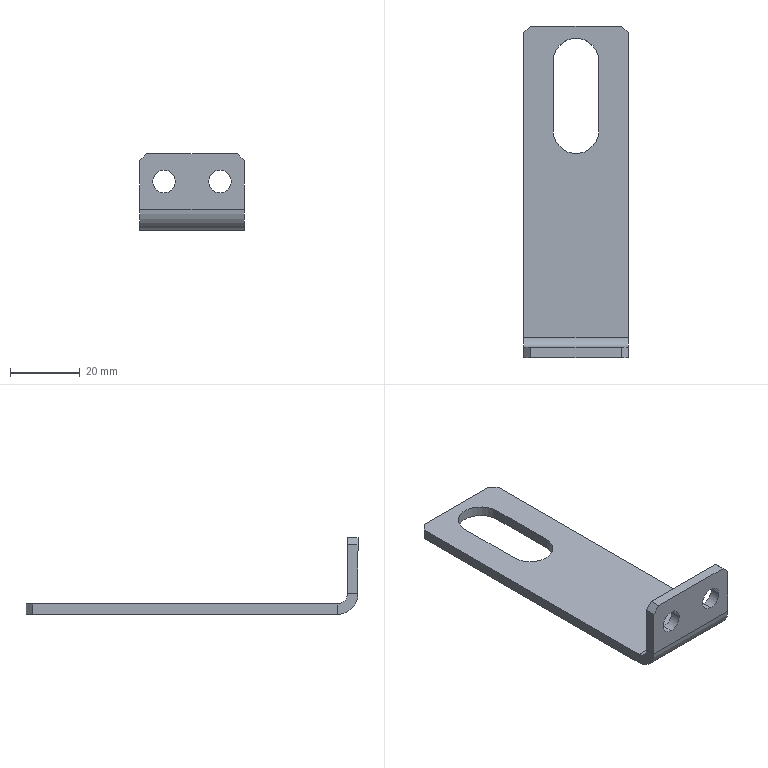Part | SolidWorks | features ICE 2, Chamfer 1, EdgeFlange 1, FlatPattern 1, SMBaseFlange 1, SheetMetal 1 | 1 solid | 26 faces | box 30 x 95 x 22 mm | volume 8685 mm3 | plane 18 | cylinder 8 | commonest cylinder face diameters 6.5 x4 13 x2 6 x1 12 x1
STEP:
#1=CARTESIAN_POINT('',(-8.,-47.5,14.25));
#2=VERTEX_POINT('',#1);
#3=CARTESIAN_POINT('',(-8.,-47.5,7.75));
#4=VERTEX_POINT('',#3);
#5=CARTESIAN_POINT('',(-8.,-47.5,11.));
#6=DIRECTION('',(0.,-1.,0.));
#7=DIRECTION('',(0.,0.,-1.));
#8=AXIS2_PLACEMENT_3D('',#5,#6,#7);
#9=CIRCLE('',#8,3.25);
#10=EDGE_CURVE('',#2,#4,#9,.T.);
#11=ORIENTED_EDGE('',*,*,#10,.T.);
#12=CARTESIAN_POINT('',(-8.,-44.5,7.75));
#13=VERTEX_POINT('',#12);
#14=CARTESIAN_POINT('',(-8.,-54.5,7.75));
#15=DIRECTION('',(0.,1.,0.));
#16=VECTOR('',#15,1000.);
#17=LINE('',#14,#16);
#18=EDGE_CURVE('',#4,#13,#17,.T.);
#19=ORIENTED_EDGE('',*,*,#18,.T.);
#20=CARTESIAN_POINT('',(-8.,-44.5,14.25));
#21=VERTEX_POINT('',#20);
#22=CARTESIAN_POINT('',(-8.,-44.5,11.));
#23=DIRECTION('',(0.,1.,0.));
#24=DIRECTION('',(0.,0.,1.));
#25=AXIS2_PLACEMENT_3D('',#22,#23,#24);
#26=CIRCLE('',#25,3.25);
#27=EDGE_CURVE('',#13,#21,#26,.T.);
#28=ORIENTED_EDGE('',*,*,#27,.T.);
#29=CARTESIAN_POINT('',(-8.,-54.5,14.25));
#30=DIRECTION('',(0.,1.,0.));
#31=VECTOR('',#30,1000.);
#32=LINE('',#29,#31);
#33=EDGE_CURVE('',#2,#21,#32,.T.);
#34=ORIENTED_EDGE('',*,*,#33,.F.);
#35=EDGE_LOOP('',(#11,#19,#28,#34));
#36=FACE_OUTER_BOUND('',#35,.T.);
#37=CARTESIAN_POINT('',(-8.,-54.5,11.));
#38=DIRECTION('',(0.,1.,0.));
#39=DIRECTION('',(0.,0.,1.));
#40=AXIS2_PLACEMENT_3D('',#37,#38,#39);
#41=CYLINDRICAL_SURFACE('',#40,3.25);
#42=ADVANCED_FACE('',(#36),#41,.F.);
#43=CARTESIAN_POINT('',(8.,-47.5,14.25));
#44=VERTEX_POINT('',#43);
#45=CARTESIAN_POINT('',(8.,-47.5,7.75));
#46=VERTEX_POINT('',#45);
#47=CARTESIAN_POINT('',(8.,-47.5,11.));
#48=DIRECTION('',(0.,-1.,0.));
#49=DIRECTION('',(0.,0.,-1.));
#50=AXIS2_PLACEMENT_3D('',#47,#48,#49);
#51=CIRCLE('',#50,3.25);
#52=EDGE_CURVE('',#44,#46,#51,.T.);
#53=ORIENTED_EDGE('',*,*,#52,.T.);
#54=CARTESIAN_POINT('',(8.,-44.5,7.75));
#55=VERTEX_POINT('',#54);
#56=CARTESIAN_POINT('',(8.,-54.5,7.75));
#57=DIRECTION('',(0.,1.,0.));
#58=VECTOR('',#57,1000.);
#59=LINE('',#56,#58);
#60=EDGE_CURVE('',#46,#55,#59,.T.);
#61=ORIENTED_EDGE('',*,*,#60,.T.);
#62=CARTESIAN_POINT('',(8.,-44.5,14.25));
#63=VERTEX_POINT('',#62);
#64=CARTESIAN_POINT('',(8.,-44.5,11.));
#65=DIRECTION('',(0.,1.,0.));
#66=DIRECTION('',(0.,0.,1.));
#67=AXIS2_PLACEMENT_3D('',#64,#65,#66);
#68=CIRCLE('',#67,3.25);
#69=EDGE_CURVE('',#55,#63,#68,.T.);
#70=ORIENTED_EDGE('',*,*,#69,.T.);
#71=CARTESIAN_POINT('',(8.,-54.5,14.25));
#72=DIRECTION('',(0.,1.,0.));
#73=VECTOR('',#72,1000.);
#74=LINE('',#71,#73);
#75=EDGE_CURVE('',#44,#63,#74,.T.);
#76=ORIENTED_EDGE('',*,*,#75,.F.);
#77=EDGE_LOOP('',(#53,#61,#70,#76));
#78=FACE_OUTER_BOUND('',#77,.T.);
#79=CARTESIAN_POINT('',(8.,-54.5,11.));
#80=DIRECTION('',(0.,1.,0.));
#81=DIRECTION('',(0.,0.,1.));
#82=AXIS2_PLACEMENT_3D('',#79,#80,#81);
#83=CYLINDRICAL_SURFACE('',#82,3.25);
#84=ADVANCED_FACE('',(#78),#83,.F.);
#85=CARTESIAN_POINT('',(15.,-41.5,-3.));
#86=VERTEX_POINT('',#85);
#87=CARTESIAN_POINT('',(15.,45.5,-3.));
#88=VERTEX_POINT('',#87);
#89=CARTESIAN_POINT('',(15.,-47.5,-3.));
#90=DIRECTION('',(0.,1.,0.));
#91=VECTOR('',#90,1000.);
#92=LINE('',#89,#91);
#93=EDGE_CURVE('',#86,#88,#92,.T.);
#94=ORIENTED_EDGE('',*,*,#93,.T.);
#95=CARTESIAN_POINT('',(15.,45.5,0.));
#96=VERTEX_POINT('',#95);
#97=CARTESIAN_POINT('',(15.,45.5,-3.));
#98=DIRECTION('',(0.,0.,1.));
#99=VECTOR('',#98,1000.);
#100=LINE('',#97,#99);
#101=EDGE_CURVE('',#88,#96,#100,.T.);
#102=ORIENTED_EDGE('',*,*,#101,.T.);
#103=CARTESIAN_POINT('',(15.,-41.5,0.));
#104=VERTEX_POINT('',#103);
#105=CARTESIAN_POINT('',(15.,-47.5,0.));
#106=DIRECTION('',(0.,1.,0.));
#107=VECTOR('',#106,1000.);
#108=LINE('',#105,#107);
#109=EDGE_CURVE('',#104,#96,#108,.T.);
#110=ORIENTED_EDGE('',*,*,#109,.F.);
#111=CARTESIAN_POINT('',(15.,-41.5,0.));
#112=DIRECTION('',(0.,0.,-1.));
#113=VECTOR('',#112,1000.);
#114=LINE('',#111,#113);
#115=EDGE_CURVE('',#104,#86,#114,.T.);
#116=ORIENTED_EDGE('',*,*,#115,.T.);
#117=EDGE_LOOP('',(#94,#102,#110,#116));
#118=FACE_OUTER_BOUND('',#117,.T.);
#119=CARTESIAN_POINT('',(15.,-47.5,-3.));
#120=DIRECTION('',(1.,0.,0.));
#121=DIRECTION('',(0.,0.,-1.));
#122=AXIS2_PLACEMENT_3D('',#119,#120,#121);
#123=PLANE('',#122);
#124=ADVANCED_FACE('',(#118),#123,.T.);
#125=CARTESIAN_POINT('',(6.5,37.5,-3.));
#126=VERTEX_POINT('',#125);
#127=CARTESIAN_POINT('',(-6.5,37.5,-3.));
#128=VERTEX_POINT('',#127);
#129=CARTESIAN_POINT('',(0.,37.5,-3.));
#130=DIRECTION('',(0.,0.,1.));
#131=DIRECTION('',(1.,0.,0.));
#132=AXIS2_PLACEMENT_3D('',#129,#130,#131);
#133=CIRCLE('',#132,6.5);
#134=EDGE_CURVE('',#126,#128,#133,.T.);
#135=ORIENTED_EDGE('',*,*,#134,.T.);
#136=CARTESIAN_POINT('',(-6.5,17.5,-3.));
#137=VERTEX_POINT('',#136);
#138=CARTESIAN_POINT('',(-6.5,37.5,-3.));
#139=DIRECTION('',(0.,-1.,0.));
#140=VECTOR('',#139,1000.);
#141=LINE('',#138,#140);
#142=EDGE_CURVE('',#128,#137,#141,.T.);
#143=ORIENTED_EDGE('',*,*,#142,.T.);
#144=CARTESIAN_POINT('',(6.5,17.5,-3.));
#145=VERTEX_POINT('',#144);
#146=CARTESIAN_POINT('',(0.,17.5,-3.));
#147=DIRECTION('',(0.,0.,1.));
#148=DIRECTION('',(1.,0.,0.));
#149=AXIS2_PLACEMENT_3D('',#146,#147,#148);
#150=CIRCLE('',#149,6.5);
#151=EDGE_CURVE('',#137,#145,#150,.T.);
#152=ORIENTED_EDGE('',*,*,#151,.T.);
#153=CARTESIAN_POINT('',(6.5,37.5,-3.));
#154=DIRECTION('',(0.,1.,0.));
#155=VECTOR('',#154,1000.);
#156=LINE('',#153,#155);
#157=EDGE_CURVE('',#145,#126,#156,.T.);
#158=ORIENTED_EDGE('',*,*,#157,.T.);
#159=EDGE_LOOP('',(#135,#143,#152,#158));
#160=FACE_BOUND('',#159,.T.);
#161=CARTESIAN_POINT('',(13.,47.5,-3.));
#162=VERTEX_POINT('',#161);
#163=CARTESIAN_POINT('',(-13.,47.5,-3.));
#164=VERTEX_POINT('',#163);
#165=CARTESIAN_POINT('',(-15.,47.5,-3.));
#166=DIRECTION('',(-1.,0.,0.));
#167=VECTOR('',#166,1000.);
#168=LINE('',#165,#167);
#169=EDGE_CURVE('',#162,#164,#168,.T.);
#170=ORIENTED_EDGE('',*,*,#169,.F.);
#171=CARTESIAN_POINT('',(30.25,30.25,-3.));
#172=DIRECTION('',(0.7071,-0.7071,0.));
#173=VECTOR('',#172,1000.);
#174=LINE('',#171,#173);
#175=EDGE_CURVE('',#162,#88,#174,.T.);
#176=ORIENTED_EDGE('',*,*,#175,.T.);
#177=ORIENTED_EDGE('',*,*,#93,.F.);
#178=CARTESIAN_POINT('',(-15.,-41.5,-3.));
#179=VERTEX_POINT('',#178);
#180=CARTESIAN_POINT('',(15.,-41.5,-3.));
#181=DIRECTION('',(-1.,0.,0.));
#182=VECTOR('',#181,1000.);
#183=LINE('',#180,#182);
#184=EDGE_CURVE('',#86,#179,#183,.T.);
#185=ORIENTED_EDGE('',*,*,#184,.T.);
#186=CARTESIAN_POINT('',(-15.,45.5,-3.));
#187=VERTEX_POINT('',#186);
#188=CARTESIAN_POINT('',(-15.,-47.5,-3.));
#189=DIRECTION('',(0.,-1.,0.));
#190=VECTOR('',#189,1000.);
#191=LINE('',#188,#190);
#192=EDGE_CURVE('',#187,#179,#191,.T.);
#193=ORIENTED_EDGE('',*,*,#192,.F.);
#194=CARTESIAN_POINT('',(-30.25,30.25,-3.));
#195=DIRECTION('',(0.7071,0.7071,0.));
#196=VECTOR('',#195,1000.);
#197=LINE('',#194,#196);
#198=EDGE_CURVE('',#187,#164,#197,.T.);
#199=ORIENTED_EDGE('',*,*,#198,.T.);
#200=EDGE_LOOP('',(#170,#176,#177,#185,#193,#199));
#201=FACE_OUTER_BOUND('',#200,.T.);
#202=CARTESIAN_POINT('',(0.,0.,-3.));
#203=DIRECTION('',(0.,0.,-1.));
#204=DIRECTION('',(-1.,0.,0.));
#205=AXIS2_PLACEMENT_3D('',#202,#203,#204);
#206=PLANE('',#205);
#207=ADVANCED_FACE('',(#160,#201),#206,.T.);
#208=CARTESIAN_POINT('',(-6.5,37.5,0.));
#209=VERTEX_POINT('',#208);
#210=CARTESIAN_POINT('',(-6.5,17.5,0.));
#211=VERTEX_POINT('',#210);
#212=CARTESIAN_POINT('',(-6.5,37.5,0.));
#213=DIRECTION('',(0.,-1.,0.));
#214=VECTOR('',#213,1000.);
#215=LINE('',#212,#214);
#216=EDGE_CURVE('',#209,#211,#215,.T.);
#217=ORIENTED_EDGE('',*,*,#216,.F.);
#218=CARTESIAN_POINT('',(6.5,37.5,0.));
#219=VERTEX_POINT('',#218);
#220=CARTESIAN_POINT('',(0.,37.5,0.));
#221=DIRECTION('',(0.,0.,1.));
#222=DIRECTION('',(1.,0.,0.));
#223=AXIS2_PLACEMENT_3D('',#220,#221,#222);
#224=CIRCLE('',#223,6.5);
#225=EDGE_CURVE('',#219,#209,#224,.T.);
#226=ORIENTED_EDGE('',*,*,#225,.F.);
#227=CARTESIAN_POINT('',(6.5,17.5,0.));
#228=VERTEX_POINT('',#227);
#229=CARTESIAN_POINT('',(6.5,37.5,0.));
#230=DIRECTION('',(0.,1.,0.));
#231=VECTOR('',#230,1000.);
#232=LINE('',#229,#231);
#233=EDGE_CURVE('',#228,#219,#232,.T.);
#234=ORIENTED_EDGE('',*,*,#233,.F.);
#235=CARTESIAN_POINT('',(0.,17.5,0.));
#236=DIRECTION('',(0.,0.,1.));
#237=DIRECTION('',(1.,0.,0.));
#238=AXIS2_PLACEMENT_3D('',#235,#236,#237);
#239=CIRCLE('',#238,6.5);
#240=EDGE_CURVE('',#211,#228,#239,.T.);
#241=ORIENTED_EDGE('',*,*,#240,.F.);
#242=EDGE_LOOP('',(#217,#226,#234,#241));
#243=FACE_BOUND('',#242,.T.);
#244=ORIENTED_EDGE('',*,*,#109,.T.);
#245=CARTESIAN_POINT('',(13.,47.5,0.));
#246=VERTEX_POINT('',#245);
#247=CARTESIAN_POINT('',(15.,45.5,0.));
#248=DIRECTION('',(-0.7071,0.7071,0.));
#249=VECTOR('',#248,1000.);
#250=LINE('',#247,#249);
#251=EDGE_CURVE('',#96,#246,#250,.T.);
#252=ORIENTED_EDGE('',*,*,#251,.T.);
#253=CARTESIAN_POINT('',(-13.,47.5,0.));
#254=VERTEX_POINT('',#253);
#255=CARTESIAN_POINT('',(-15.,47.5,0.));
#256=DIRECTION('',(-1.,0.,0.));
#257=VECTOR('',#256,1000.);
#258=LINE('',#255,#257);
#259=EDGE_CURVE('',#246,#254,#258,.T.);
#260=ORIENTED_EDGE('',*,*,#259,.T.);
#261=CARTESIAN_POINT('',(-15.,45.5,0.));
#262=VERTEX_POINT('',#261);
#263=CARTESIAN_POINT('',(-13.,47.5,0.));
#264=DIRECTION('',(-0.7071,-0.7071,0.));
#265=VECTOR('',#264,1000.);
#266=LINE('',#263,#265);
#267=EDGE_CURVE('',#254,#262,#266,.T.);
#268=ORIENTED_EDGE('',*,*,#267,.T.);
#269=CARTESIAN_POINT('',(-15.,-41.5,0.));
#270=VERTEX_POINT('',#269);
#271=CARTESIAN_POINT('',(-15.,-47.5,0.));
#272=DIRECTION('',(0.,-1.,0.));
#273=VECTOR('',#272,1000.);
#274=LINE('',#271,#273);
#275=EDGE_CURVE('',#262,#270,#274,.T.);
#276=ORIENTED_EDGE('',*,*,#275,.T.);
#277=CARTESIAN_POINT('',(15.,-41.5,0.));
#278=DIRECTION('',(-1.,0.,0.));
#279=VECTOR('',#278,1000.);
#280=LINE('',#277,#279);
#281=EDGE_CURVE('',#104,#270,#280,.T.);
#282=ORIENTED_EDGE('',*,*,#281,.F.);
#283=EDGE_LOOP('',(#244,#252,#260,#268,#276,#282));
#284=FACE_OUTER_BOUND('',#283,.T.);
#285=CARTESIAN_POINT('',(0.,0.,0.));
#286=DIRECTION('',(0.,0.,-1.));
#287=DIRECTION('',(-1.,0.,0.));
#288=AXIS2_PLACEMENT_3D('',#285,#286,#287);
#289=PLANE('',#288);
#290=ADVANCED_FACE('',(#243,#284),#289,.F.);
#291=ORIENTED_EDGE('',*,*,#275,.F.);
#292=CARTESIAN_POINT('',(-15.,45.5,-3.));
#293=DIRECTION('',(0.,0.,-1.));
#294=VECTOR('',#293,1000.);
#295=LINE('',#292,#294);
#296=EDGE_CURVE('',#262,#187,#295,.T.);
#297=ORIENTED_EDGE('',*,*,#296,.T.);
#298=ORIENTED_EDGE('',*,*,#192,.T.);
#299=CARTESIAN_POINT('',(-15.,-41.5,0.));
#300=DIRECTION('',(0.,0.,-1.));
#301=VECTOR('',#300,1000.);
#302=LINE('',#299,#301);
#303=EDGE_CURVE('',#270,#179,#302,.T.);
#304=ORIENTED_EDGE('',*,*,#303,.F.);
#305=EDGE_LOOP('',(#291,#297,#298,#304));
#306=FACE_OUTER_BOUND('',#305,.T.);
#307=CARTESIAN_POINT('',(-15.,-47.5,-3.));
#308=DIRECTION('',(-1.,0.,0.));
#309=DIRECTION('',(0.,0.,1.));
#310=AXIS2_PLACEMENT_3D('',#307,#308,#309);
#311=PLANE('',#310);
#312=ADVANCED_FACE('',(#306),#311,.T.);
#313=ORIENTED_EDGE('',*,*,#259,.F.);
#314=CARTESIAN_POINT('',(13.,47.5,-3.));
#315=DIRECTION('',(0.,0.,-1.));
#316=VECTOR('',#315,1000.);
#317=LINE('',#314,#316);
#318=EDGE_CURVE('',#246,#162,#317,.T.);
#319=ORIENTED_EDGE('',*,*,#318,.T.);
#320=ORIENTED_EDGE('',*,*,#169,.T.);
#321=CARTESIAN_POINT('',(-13.,47.5,-3.));
#322=DIRECTION('',(0.,0.,1.));
#323=VECTOR('',#322,1000.);
#324=LINE('',#321,#323);
#325=EDGE_CURVE('',#164,#254,#324,.T.);
#326=ORIENTED_EDGE('',*,*,#325,.T.);
#327=EDGE_LOOP('',(#313,#319,#320,#326));
#328=FACE_OUTER_BOUND('',#327,.T.);
#329=CARTESIAN_POINT('',(-15.,47.5,-3.));
#330=DIRECTION('',(0.,1.,0.));
#331=DIRECTION('',(0.,0.,1.));
#332=AXIS2_PLACEMENT_3D('',#329,#330,#331);
#333=PLANE('',#332);
#334=ADVANCED_FACE('',(#328),#333,.T.);
#335=CARTESIAN_POINT('',(-15.,-44.5,3.));
#336=VERTEX_POINT('',#335);
#337=CARTESIAN_POINT('',(-15.,-47.5,3.));
#338=VERTEX_POINT('',#337);
#339=CARTESIAN_POINT('',(-15.,-47.5,3.));
#340=DIRECTION('',(0.,-1.,0.));
#341=VECTOR('',#340,1000.);
#342=LINE('',#339,#341);
#343=EDGE_CURVE('',#336,#338,#342,.T.);
#344=ORIENTED_EDGE('',*,*,#343,.F.);
#345=CARTESIAN_POINT('',(-15.,-41.5,3.));
#346=DIRECTION('',(-1.,0.,0.));
#347=DIRECTION('',(0.,0.,-1.));
#348=AXIS2_PLACEMENT_3D('',#345,#346,#347);
#349=CIRCLE('',#348,3.);
#350=EDGE_CURVE('',#270,#336,#349,.T.);
#351=ORIENTED_EDGE('',*,*,#350,.F.);
#352=ORIENTED_EDGE('',*,*,#303,.T.);
#353=CARTESIAN_POINT('',(-15.,-41.5,3.));
#354=DIRECTION('',(-1.,0.,0.));
#355=DIRECTION('',(0.,0.,-1.));
#356=AXIS2_PLACEMENT_3D('',#353,#354,#355);
#357=CIRCLE('',#356,6.);
#358=EDGE_CURVE('',#179,#338,#357,.T.);
#359=ORIENTED_EDGE('',*,*,#358,.T.);
#360=EDGE_LOOP('',(#344,#351,#352,#359));
#361=FACE_OUTER_BOUND('',#360,.T.);
#362=CARTESIAN_POINT('',(-15.,-41.5,3.));
#363=DIRECTION('',(-1.,0.,0.));
#364=DIRECTION('',(0.,0.,1.));
#365=AXIS2_PLACEMENT_3D('',#362,#363,#364);
#366=PLANE('',#365);
#367=ADVANCED_FACE('',(#361),#366,.T.);
#368=CARTESIAN_POINT('',(15.,-44.5,3.));
#369=VERTEX_POINT('',#368);
#370=CARTESIAN_POINT('',(15.,-41.5,3.));
#371=DIRECTION('',(1.,0.,0.));
#372=DIRECTION('',(0.,0.,-1.));
#373=AXIS2_PLACEMENT_3D('',#370,#371,#372);
#374=CIRCLE('',#373,3.);
#375=EDGE_CURVE('',#369,#104,#374,.T.);
#376=ORIENTED_EDGE('',*,*,#375,.F.);
#377=CARTESIAN_POINT('',(15.,-47.5,3.));
#378=VERTEX_POINT('',#377);
#379=CARTESIAN_POINT('',(15.,-44.5,3.));
#380=DIRECTION('',(0.,-1.,0.));
#381=VECTOR('',#380,1000.);
#382=LINE('',#379,#381);
#383=EDGE_CURVE('',#369,#378,#382,.T.);
#384=ORIENTED_EDGE('',*,*,#383,.T.);
#385=CARTESIAN_POINT('',(15.,-41.5,3.));
#386=DIRECTION('',(1.,0.,0.));
#387=DIRECTION('',(0.,0.,-1.));
#388=AXIS2_PLACEMENT_3D('',#385,#386,#387);
#389=CIRCLE('',#388,6.);
#390=EDGE_CURVE('',#378,#86,#389,.T.);
#391=ORIENTED_EDGE('',*,*,#390,.T.);
#392=ORIENTED_EDGE('',*,*,#115,.F.);
#393=EDGE_LOOP('',(#376,#384,#391,#392));
#394=FACE_OUTER_BOUND('',#393,.T.);
#395=CARTESIAN_POINT('',(15.,-41.5,3.));
#396=DIRECTION('',(-1.,0.,0.));
#397=DIRECTION('',(0.,0.,1.));
#398=AXIS2_PLACEMENT_3D('',#395,#396,#397);
#399=PLANE('',#398);
#400=ADVANCED_FACE('',(#394),#399,.F.);
#401=ORIENTED_EDGE('',*,*,#184,.F.);
#402=ORIENTED_EDGE('',*,*,#390,.F.);
#403=CARTESIAN_POINT('',(0.,-47.5,3.));
#404=DIRECTION('',(1.,0.,0.));
#405=VECTOR('',#404,1000.);
#406=LINE('',#403,#405);
#407=EDGE_CURVE('',#338,#378,#406,.T.);
#408=ORIENTED_EDGE('',*,*,#407,.F.);
#409=ORIENTED_EDGE('',*,*,#358,.F.);
#410=EDGE_LOOP('',(#401,#402,#408,#409));
#411=FACE_OUTER_BOUND('',#410,.T.);
#412=CARTESIAN_POINT('',(15.,-41.5,3.));
#413=DIRECTION('',(1.,0.,0.));
#414=DIRECTION('',(0.,-1.,0.));
#415=AXIS2_PLACEMENT_3D('',#412,#413,#414);
#416=CYLINDRICAL_SURFACE('',#415,6.);
#417=ADVANCED_FACE('',(#411),#416,.T.);
#418=ORIENTED_EDGE('',*,*,#281,.T.);
#419=ORIENTED_EDGE('',*,*,#350,.T.);
#420=CARTESIAN_POINT('',(-15.,-44.5,3.));
#421=DIRECTION('',(1.,0.,0.));
#422=VECTOR('',#421,1000.);
#423=LINE('',#420,#422);
#424=EDGE_CURVE('',#336,#369,#423,.T.);
#425=ORIENTED_EDGE('',*,*,#424,.T.);
#426=ORIENTED_EDGE('',*,*,#375,.T.);
#427=EDGE_LOOP('',(#418,#419,#425,#426));
#428=FACE_OUTER_BOUND('',#427,.T.);
#429=CARTESIAN_POINT('',(15.,-41.5,3.));
#430=DIRECTION('',(1.,0.,0.));
#431=DIRECTION('',(0.,-1.,0.));
#432=AXIS2_PLACEMENT_3D('',#429,#430,#431);
#433=CYLINDRICAL_SURFACE('',#432,3.);
#434=ADVANCED_FACE('',(#428),#433,.F.);
#435=CARTESIAN_POINT('',(15.,-44.5,17.));
#436=VERTEX_POINT('',#435);
#437=CARTESIAN_POINT('',(15.,-44.5,0.));
#438=DIRECTION('',(0.,0.,-1.));
#439=VECTOR('',#438,1000.);
#440=LINE('',#437,#439);
#441=EDGE_CURVE('',#436,#369,#440,.T.);
#442=ORIENTED_EDGE('',*,*,#441,.F.);
#443=CARTESIAN_POINT('',(15.,-47.5,17.));
#444=VERTEX_POINT('',#443);
#445=CARTESIAN_POINT('',(15.,-47.5,17.));
#446=DIRECTION('',(0.,-1.,0.));
#447=VECTOR('',#446,1000.);
#448=LINE('',#445,#447);
#449=EDGE_CURVE('',#436,#444,#448,.T.);
#450=ORIENTED_EDGE('',*,*,#449,.T.);
#451=CARTESIAN_POINT('',(15.,-47.5,0.));
#452=DIRECTION('',(0.,0.,-1.));
#453=VECTOR('',#452,1000.);
#454=LINE('',#451,#453);
#455=EDGE_CURVE('',#444,#378,#454,.T.);
#456=ORIENTED_EDGE('',*,*,#455,.T.);
#457=ORIENTED_EDGE('',*,*,#383,.F.);
#458=EDGE_LOOP('',(#442,#450,#456,#457));
#459=FACE_OUTER_BOUND('',#458,.T.);
#460=CARTESIAN_POINT('',(15.,-47.5,0.));
#461=DIRECTION('',(1.,0.,0.));
#462=DIRECTION('',(0.,0.,-1.));
#463=AXIS2_PLACEMENT_3D('',#460,#461,#462);
#464=PLANE('',#463);
#465=ADVANCED_FACE('',(#459),#464,.T.);
#466=CARTESIAN_POINT('',(-15.,-47.5,17.));
#467=VERTEX_POINT('',#466);
#468=CARTESIAN_POINT('',(-15.,-47.5,19.));
#469=DIRECTION('',(0.,0.,1.));
#470=VECTOR('',#469,1000.);
#471=LINE('',#468,#470);
#472=EDGE_CURVE('',#338,#467,#471,.T.);
#473=ORIENTED_EDGE('',*,*,#472,.T.);
#474=CARTESIAN_POINT('',(-15.,-44.5,17.));
#475=VERTEX_POINT('',#474);
#476=CARTESIAN_POINT('',(-15.,-47.5,17.));
#477=DIRECTION('',(0.,1.,0.));
#478=VECTOR('',#477,1000.);
#479=LINE('',#476,#478);
#480=EDGE_CURVE('',#467,#475,#479,.T.);
#481=ORIENTED_EDGE('',*,*,#480,.T.);
#482=CARTESIAN_POINT('',(-15.,-44.5,0.));
#483=DIRECTION('',(0.,0.,1.));
#484=VECTOR('',#483,1000.);
#485=LINE('',#482,#484);
#486=EDGE_CURVE('',#336,#475,#485,.T.);
#487=ORIENTED_EDGE('',*,*,#486,.F.);
#488=ORIENTED_EDGE('',*,*,#343,.T.);
#489=EDGE_LOOP('',(#473,#481,#487,#488));
#490=FACE_OUTER_BOUND('',#489,.T.);
#491=CARTESIAN_POINT('',(-15.,-47.5,19.));
#492=DIRECTION('',(-1.,0.,0.));
#493=DIRECTION('',(0.,0.,1.));
#494=AXIS2_PLACEMENT_3D('',#491,#492,#493);
#495=PLANE('',#494);
#496=ADVANCED_FACE('',(#490),#495,.T.);
#497=ORIENTED_EDGE('',*,*,#10,.F.);
#498=CARTESIAN_POINT('',(-8.,-47.5,11.));
#499=DIRECTION('',(0.,-1.,0.));
#500=DIRECTION('',(0.,0.,-1.));
#501=AXIS2_PLACEMENT_3D('',#498,#499,#500);
#502=CIRCLE('',#501,3.25);
#503=EDGE_CURVE('',#4,#2,#502,.T.);
#504=ORIENTED_EDGE('',*,*,#503,.F.);
#505=EDGE_LOOP('',(#497,#504));
#506=FACE_BOUND('',#505,.T.);
#507=ORIENTED_EDGE('',*,*,#52,.F.);
#508=CARTESIAN_POINT('',(8.,-47.5,11.));
#509=DIRECTION('',(0.,-1.,0.));
#510=DIRECTION('',(0.,0.,-1.));
#511=AXIS2_PLACEMENT_3D('',#508,#509,#510);
#512=CIRCLE('',#511,3.25);
#513=EDGE_CURVE('',#46,#44,#512,.T.);
#514=ORIENTED_EDGE('',*,*,#513,.F.);
#515=EDGE_LOOP('',(#507,#514));
#516=FACE_BOUND('',#515,.T.);
#517=ORIENTED_EDGE('',*,*,#455,.F.);
#518=CARTESIAN_POINT('',(13.,-47.5,19.));
#519=VERTEX_POINT('',#518);
#520=CARTESIAN_POINT('',(16.,-47.5,16.));
#521=DIRECTION('',(-0.7071,0.,0.7071));
#522=VECTOR('',#521,1000.);
#523=LINE('',#520,#522);
#524=EDGE_CURVE('',#444,#519,#523,.T.);
#525=ORIENTED_EDGE('',*,*,#524,.T.);
#526=CARTESIAN_POINT('',(-13.,-47.5,19.));
#527=VERTEX_POINT('',#526);
#528=CARTESIAN_POINT('',(15.,-47.5,19.));
#529=DIRECTION('',(1.,0.,0.));
#530=VECTOR('',#529,1000.);
#531=LINE('',#528,#530);
#532=EDGE_CURVE('',#527,#519,#531,.T.);
#533=ORIENTED_EDGE('',*,*,#532,.F.);
#534=CARTESIAN_POINT('',(-16.,-47.5,16.));
#535=DIRECTION('',(-0.7071,0.,-0.7071));
#536=VECTOR('',#535,1000.);
#537=LINE('',#534,#536);
#538=EDGE_CURVE('',#527,#467,#537,.T.);
#539=ORIENTED_EDGE('',*,*,#538,.T.);
#540=ORIENTED_EDGE('',*,*,#472,.F.);
#541=ORIENTED_EDGE('',*,*,#407,.T.);
#542=EDGE_LOOP('',(#517,#525,#533,#539,#540,#541));
#543=FACE_OUTER_BOUND('',#542,.T.);
#544=CARTESIAN_POINT('',(0.,-47.5,0.));
#545=DIRECTION('',(0.,-1.,0.));
#546=DIRECTION('',(0.,0.,-1.));
#547=AXIS2_PLACEMENT_3D('',#544,#545,#546);
#548=PLANE('',#547);
#549=ADVANCED_FACE('',(#506,#516,#543),#548,.T.);
#550=CARTESIAN_POINT('',(-8.,-44.5,11.));
#551=DIRECTION('',(0.,1.,0.));
#552=DIRECTION('',(0.,0.,1.));
#553=AXIS2_PLACEMENT_3D('',#550,#551,#552);
#554=CIRCLE('',#553,3.25);
#555=EDGE_CURVE('',#21,#13,#554,.T.);
#556=ORIENTED_EDGE('',*,*,#555,.F.);
#557=ORIENTED_EDGE('',*,*,#27,.F.);
#558=EDGE_LOOP('',(#556,#557));
#559=FACE_BOUND('',#558,.T.);
#560=CARTESIAN_POINT('',(8.,-44.5,11.));
#561=DIRECTION('',(0.,1.,0.));
#562=DIRECTION('',(0.,0.,1.));
#563=AXIS2_PLACEMENT_3D('',#560,#561,#562);
#564=CIRCLE('',#563,3.25);
#565=EDGE_CURVE('',#63,#55,#564,.T.);
#566=ORIENTED_EDGE('',*,*,#565,.F.);
#567=ORIENTED_EDGE('',*,*,#69,.F.);
#568=EDGE_LOOP('',(#566,#567));
#569=FACE_BOUND('',#568,.T.);
#570=CARTESIAN_POINT('',(-13.,-44.5,19.));
#571=VERTEX_POINT('',#570);
#572=CARTESIAN_POINT('',(13.,-44.5,19.));
#573=VERTEX_POINT('',#572);
#574=CARTESIAN_POINT('',(0.,-44.5,19.));
#575=DIRECTION('',(1.,0.,0.));
#576=VECTOR('',#575,1000.);
#577=LINE('',#574,#576);
#578=EDGE_CURVE('',#571,#573,#577,.T.);
#579=ORIENTED_EDGE('',*,*,#578,.T.);
#580=CARTESIAN_POINT('',(13.,-44.5,19.));
#581=DIRECTION('',(0.7071,0.,-0.7071));
#582=VECTOR('',#581,1000.);
#583=LINE('',#580,#582);
#584=EDGE_CURVE('',#573,#436,#583,.T.);
#585=ORIENTED_EDGE('',*,*,#584,.T.);
#586=ORIENTED_EDGE('',*,*,#441,.T.);
#587=ORIENTED_EDGE('',*,*,#424,.F.);
#588=ORIENTED_EDGE('',*,*,#486,.T.);
#589=CARTESIAN_POINT('',(-15.,-44.5,17.));
#590=DIRECTION('',(0.7071,0.,0.7071));
#591=VECTOR('',#590,1000.);
#592=LINE('',#589,#591);
#593=EDGE_CURVE('',#475,#571,#592,.T.);
#594=ORIENTED_EDGE('',*,*,#593,.T.);
#595=EDGE_LOOP('',(#579,#585,#586,#587,#588,#594));
#596=FACE_OUTER_BOUND('',#595,.T.);
#597=CARTESIAN_POINT('',(0.,-44.5,0.));
#598=DIRECTION('',(0.,-1.,0.));
#599=DIRECTION('',(0.,0.,-1.));
#600=AXIS2_PLACEMENT_3D('',#597,#598,#599);
#601=PLANE('',#600);
#602=ADVANCED_FACE('',(#559,#569,#596),#601,.F.);
#603=ORIENTED_EDGE('',*,*,#532,.T.);
#604=CARTESIAN_POINT('',(13.,-47.5,19.));
#605=DIRECTION('',(0.,1.,0.));
#606=VECTOR('',#605,1000.);
#607=LINE('',#604,#606);
#608=EDGE_CURVE('',#519,#573,#607,.T.);
#609=ORIENTED_EDGE('',*,*,#608,.T.);
#610=ORIENTED_EDGE('',*,*,#578,.F.);
#611=CARTESIAN_POINT('',(-13.,-47.5,19.));
#612=DIRECTION('',(0.,-1.,0.));
#613=VECTOR('',#612,1000.);
#614=LINE('',#611,#613);
#615=EDGE_CURVE('',#571,#527,#614,.T.);
#616=ORIENTED_EDGE('',*,*,#615,.T.);
#617=EDGE_LOOP('',(#603,#609,#610,#616));
#618=FACE_OUTER_BOUND('',#617,.T.);
#619=CARTESIAN_POINT('',(15.,-47.5,19.));
#620=DIRECTION('',(0.,0.,1.));
#621=DIRECTION('',(0.,-1.,0.));
#622=AXIS2_PLACEMENT_3D('',#619,#620,#621);
#623=PLANE('',#622);
#624=ADVANCED_FACE('',(#618),#623,.T.);
#625=ORIENTED_EDGE('',*,*,#524,.F.);
#626=ORIENTED_EDGE('',*,*,#449,.F.);
#627=ORIENTED_EDGE('',*,*,#584,.F.);
#628=ORIENTED_EDGE('',*,*,#608,.F.);
#629=EDGE_LOOP('',(#625,#626,#627,#628));
#630=FACE_OUTER_BOUND('',#629,.T.);
#631=CARTESIAN_POINT('',(13.,-47.5,19.));
#632=DIRECTION('',(-0.7071,0.,-0.7071));
#633=DIRECTION('',(0.,1.,0.));
#634=AXIS2_PLACEMENT_3D('',#631,#632,#633);
#635=PLANE('',#634);
#636=ADVANCED_FACE('',(#630),#635,.F.);
#637=ORIENTED_EDGE('',*,*,#538,.F.);
#638=ORIENTED_EDGE('',*,*,#615,.F.);
#639=ORIENTED_EDGE('',*,*,#593,.F.);
#640=ORIENTED_EDGE('',*,*,#480,.F.);
#641=EDGE_LOOP('',(#637,#638,#639,#640));
#642=FACE_OUTER_BOUND('',#641,.T.);
#643=CARTESIAN_POINT('',(-15.,-47.5,17.));
#644=DIRECTION('',(0.7071,0.,-0.7071));
#645=DIRECTION('',(0.,1.,0.));
#646=AXIS2_PLACEMENT_3D('',#643,#644,#645);
#647=PLANE('',#646);
#648=ADVANCED_FACE('',(#642),#647,.F.);
#649=ORIENTED_EDGE('',*,*,#175,.F.);
#650=ORIENTED_EDGE('',*,*,#318,.F.);
#651=ORIENTED_EDGE('',*,*,#251,.F.);
#652=ORIENTED_EDGE('',*,*,#101,.F.);
#653=EDGE_LOOP('',(#649,#650,#651,#652));
#654=FACE_OUTER_BOUND('',#653,.T.);
#655=CARTESIAN_POINT('',(15.,45.5,-3.));
#656=DIRECTION('',(-0.7071,-0.7071,0.));
#657=DIRECTION('',(0.,0.,1.));
#658=AXIS2_PLACEMENT_3D('',#655,#656,#657);
#659=PLANE('',#658);
#660=ADVANCED_FACE('',(#654),#659,.F.);
#661=ORIENTED_EDGE('',*,*,#198,.F.);
#662=ORIENTED_EDGE('',*,*,#296,.F.);
#663=ORIENTED_EDGE('',*,*,#267,.F.);
#664=ORIENTED_EDGE('',*,*,#325,.F.);
#665=EDGE_LOOP('',(#661,#662,#663,#664));
#666=FACE_OUTER_BOUND('',#665,.T.);
#667=CARTESIAN_POINT('',(-13.,47.5,-3.));
#668=DIRECTION('',(0.7071,-0.7071,0.));
#669=DIRECTION('',(0.,0.,1.));
#670=AXIS2_PLACEMENT_3D('',#667,#668,#669);
#671=PLANE('',#670);
#672=ADVANCED_FACE('',(#666),#671,.F.);
#673=ORIENTED_EDGE('',*,*,#225,.T.);
#674=CARTESIAN_POINT('',(-6.5,37.5,-3.));
#675=DIRECTION('',(0.,0.,1.));
#676=VECTOR('',#675,1000.);
#677=LINE('',#674,#676);
#678=EDGE_CURVE('',#128,#209,#677,.T.);
#679=ORIENTED_EDGE('',*,*,#678,.F.);
#680=ORIENTED_EDGE('',*,*,#134,.F.);
#681=CARTESIAN_POINT('',(6.5,37.5,-3.));
#682=DIRECTION('',(0.,0.,1.));
#683=VECTOR('',#682,1000.);
#684=LINE('',#681,#683);
#685=EDGE_CURVE('',#126,#219,#684,.T.);
#686=ORIENTED_EDGE('',*,*,#685,.T.);
#687=EDGE_LOOP('',(#673,#679,#680,#686));
#688=FACE_OUTER_BOUND('',#687,.T.);
#689=CARTESIAN_POINT('',(0.,37.5,-3.));
#690=DIRECTION('',(0.,0.,1.));
#691=DIRECTION('',(1.,0.,0.));
#692=AXIS2_PLACEMENT_3D('',#689,#690,#691);
#693=CYLINDRICAL_SURFACE('',#692,6.5);
#694=ADVANCED_FACE('',(#688),#693,.F.);
#695=ORIENTED_EDGE('',*,*,#233,.T.);
#696=ORIENTED_EDGE('',*,*,#685,.F.);
#697=ORIENTED_EDGE('',*,*,#157,.F.);
#698=CARTESIAN_POINT('',(6.5,17.5,-3.));
#699=DIRECTION('',(0.,0.,1.));
#700=VECTOR('',#699,1000.);
#701=LINE('',#698,#700);
#702=EDGE_CURVE('',#145,#228,#701,.T.);
#703=ORIENTED_EDGE('',*,*,#702,.T.);
#704=EDGE_LOOP('',(#695,#696,#697,#703));
#705=FACE_OUTER_BOUND('',#704,.T.);
#706=CARTESIAN_POINT('',(6.5,37.5,-3.));
#707=DIRECTION('',(1.,0.,0.));
#708=DIRECTION('',(0.,1.,0.));
#709=AXIS2_PLACEMENT_3D('',#706,#707,#708);
#710=PLANE('',#709);
#711=ADVANCED_FACE('',(#705),#710,.F.);
#712=ORIENTED_EDGE('',*,*,#240,.T.);
#713=ORIENTED_EDGE('',*,*,#702,.F.);
#714=ORIENTED_EDGE('',*,*,#151,.F.);
#715=CARTESIAN_POINT('',(-6.5,17.5,-3.));
#716=DIRECTION('',(0.,0.,1.));
#717=VECTOR('',#716,1000.);
#718=LINE('',#715,#717);
#719=EDGE_CURVE('',#137,#211,#718,.T.);
#720=ORIENTED_EDGE('',*,*,#719,.T.);
#721=EDGE_LOOP('',(#712,#713,#714,#720));
#722=FACE_OUTER_BOUND('',#721,.T.);
#723=CARTESIAN_POINT('',(0.,17.5,-3.));
#724=DIRECTION('',(0.,0.,1.));
#725=DIRECTION('',(1.,0.,0.));
#726=AXIS2_PLACEMENT_3D('',#723,#724,#725);
#727=CYLINDRICAL_SURFACE('',#726,6.5);
#728=ADVANCED_FACE('',(#722),#727,.F.);
#729=ORIENTED_EDGE('',*,*,#216,.T.);
#730=ORIENTED_EDGE('',*,*,#719,.F.);
#731=ORIENTED_EDGE('',*,*,#142,.F.);
#732=ORIENTED_EDGE('',*,*,#678,.T.);
#733=EDGE_LOOP('',(#729,#730,#731,#732));
#734=FACE_OUTER_BOUND('',#733,.T.);
#735=CARTESIAN_POINT('',(-6.5,37.5,-3.));
#736=DIRECTION('',(-1.,0.,0.));
#737=DIRECTION('',(0.,-1.,0.));
#738=AXIS2_PLACEMENT_3D('',#735,#736,#737);
#739=PLANE('',#738);
#740=ADVANCED_FACE('',(#734),#739,.F.);
#741=ORIENTED_EDGE('',*,*,#60,.F.);
#742=ORIENTED_EDGE('',*,*,#513,.T.);
#743=ORIENTED_EDGE('',*,*,#75,.T.);
#744=ORIENTED_EDGE('',*,*,#565,.T.);
#745=EDGE_LOOP('',(#741,#742,#743,#744));
#746=FACE_OUTER_BOUND('',#745,.T.);
#747=CARTESIAN_POINT('',(8.,-54.5,11.));
#748=DIRECTION('',(0.,1.,0.));
#749=DIRECTION('',(0.,0.,1.));
#750=AXIS2_PLACEMENT_3D('',#747,#748,#749);
#751=CYLINDRICAL_SURFACE('',#750,3.25);
#752=ADVANCED_FACE('',(#746),#751,.F.);
#753=ORIENTED_EDGE('',*,*,#18,.F.);
#754=ORIENTED_EDGE('',*,*,#503,.T.);
#755=ORIENTED_EDGE('',*,*,#33,.T.);
#756=ORIENTED_EDGE('',*,*,#555,.T.);
#757=EDGE_LOOP('',(#753,#754,#755,#756));
#758=FACE_OUTER_BOUND('',#757,.T.);
#759=CARTESIAN_POINT('',(-8.,-54.5,11.));
#760=DIRECTION('',(0.,1.,0.));
#761=DIRECTION('',(0.,0.,1.));
#762=AXIS2_PLACEMENT_3D('',#759,#760,#761);
#763=CYLINDRICAL_SURFACE('',#762,3.25);
#764=ADVANCED_FACE('',(#758),#763,.F.);
#765=CLOSED_SHELL('',(#42,#84,#124,#207,#290,#312,#334,#367,#400,#417,#434,#465,#496,#549,#602,#624,#636,#648,#660,#672,#694,#711,#728,#740,#752,#764));
#766=MANIFOLD_SOLID_BREP('',#765);
#767=CARTESIAN_POINT('',(0.,0.,0.));
#768=DIRECTION('',(0.,0.,1.));
#769=DIRECTION('',(1.,0.,0.));
#770=AXIS2_PLACEMENT_3D('',#767,#768,#769);
#771=(LENGTH_UNIT()NAMED_UNIT(*)SI_UNIT(.MILLI.,.METRE.));
#772=UNCERTAINTY_MEASURE_WITH_UNIT(LENGTH_MEASURE(0.00001),#771,'','');
#773=(NAMED_UNIT(*)PLANE_ANGLE_UNIT()SI_UNIT($,.RADIAN.));
#774=(NAMED_UNIT(*)SI_UNIT($,.STERADIAN.)SOLID_ANGLE_UNIT());
#775=(GEOMETRIC_REPRESENTATION_CONTEXT(3)GLOBAL_UNCERTAINTY_ASSIGNED_CONTEXT((#772))GLOBAL_UNIT_ASSIGNED_CONTEXT((#771,#773,#774))REPRESENTATION_CONTEXT('',''));
#776=ADVANCED_BREP_SHAPE_REPRESENTATION('',(#766,#770),#775);